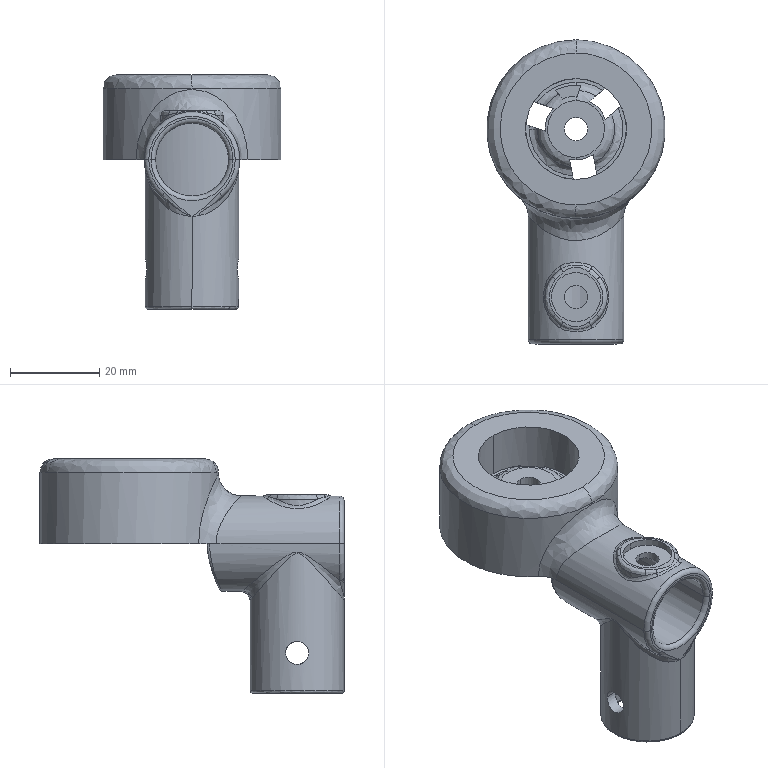Part | SolidWorks | features BaseBody 1 | 1 solid | 239 faces | box 40 x 68.161 x 52.5 mm | volume 24103 mm3 | spline 124 | cylinder 72 | plane 37 | torus 5 | cone 1 | commonest cylinder face diameters 1 x15 34.6 x13 5.2 x8 16.176 x4 13.8 x3 0.078 x2